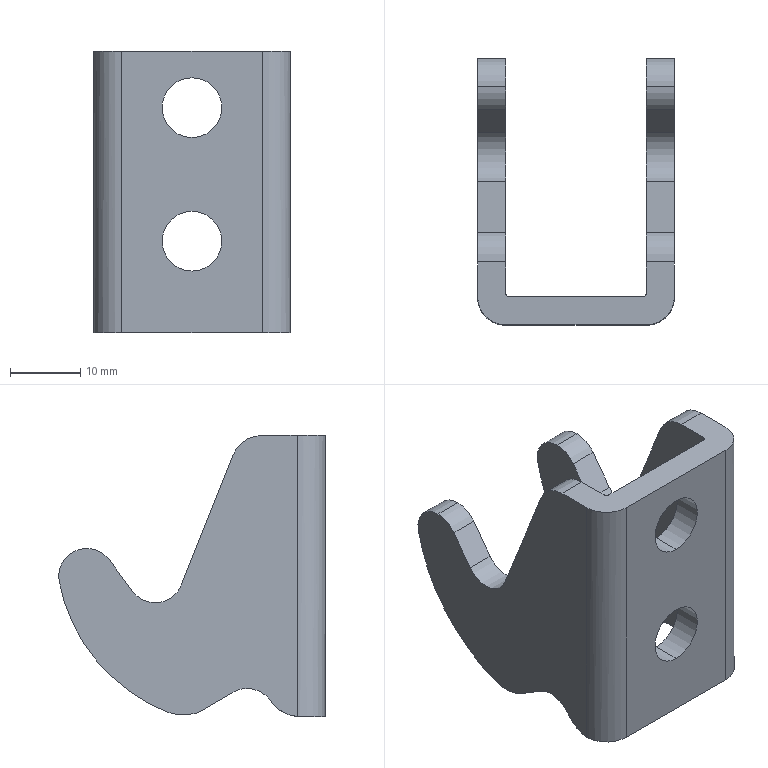Part | STEP file | _4-QC-408710.step | 1 solid | 41 faces | box 28 x 37.92 x 40 mm | volume 9998 mm3 | cylinder 25 | plane 16 | commonest cylinder face diameters 8 x12 8.5 x4 1 x2 9 x2 12 x2 50 x2